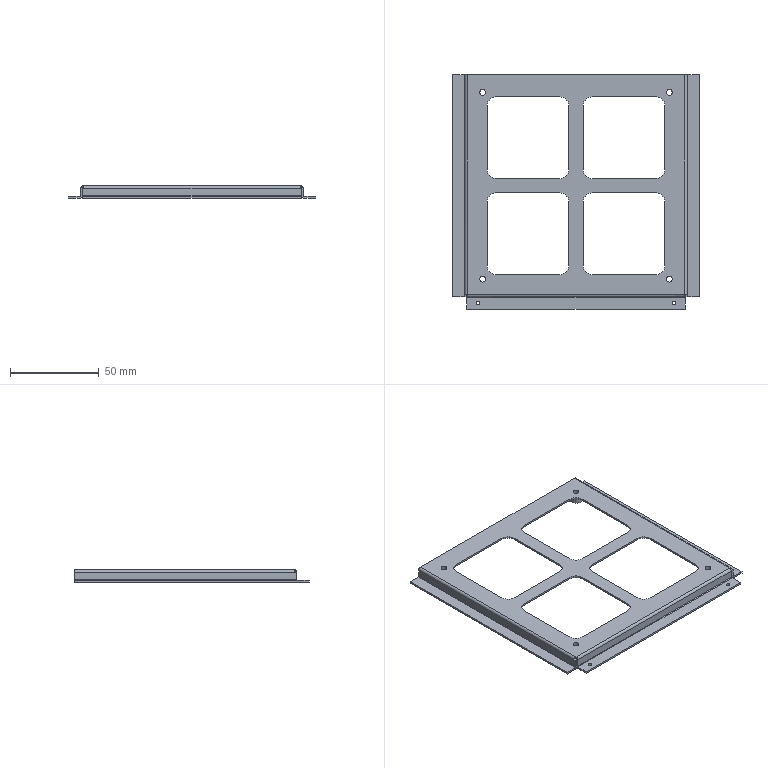Part | STEP file | FHD-021-004-B fan support cover | 1 solid | 88 faces | box 139 x 132 x 7 mm | volume 12460 mm3 | plane 46 | cylinder 38 | spline 4 | commonest cylinder face diameters 10 x16 0.6 x6 2.6 x6 3.3 x4 8 x4 2 x2